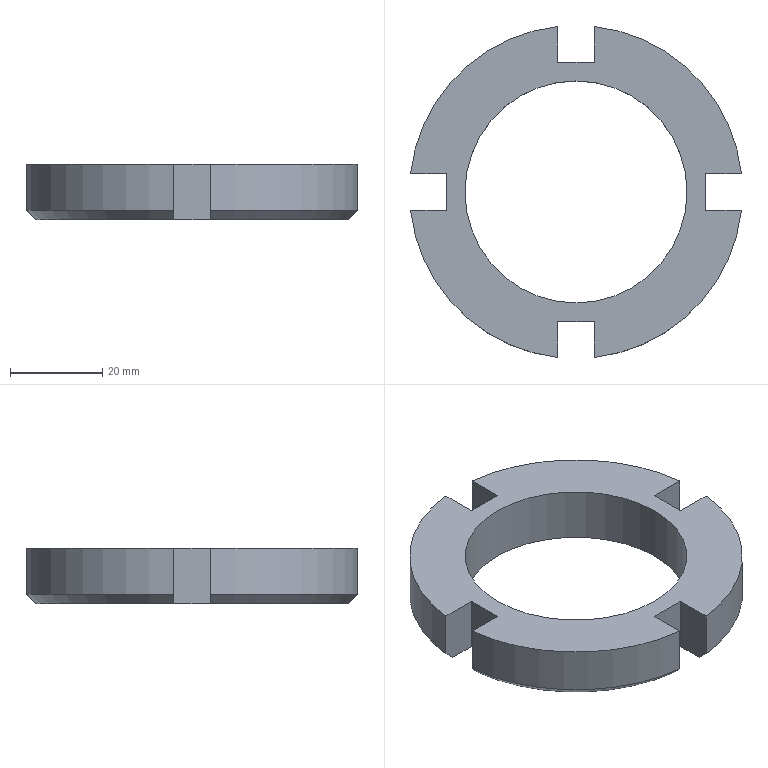Part | STEP file | M42 nut | 1 solid | 24 faces | box 71.554 x 71.554 x 12 mm | volume 23720 mm3 | plane 14 | cylinder 6 | cone 4 | commonest cylinder face diameters 72 x4 48 x2